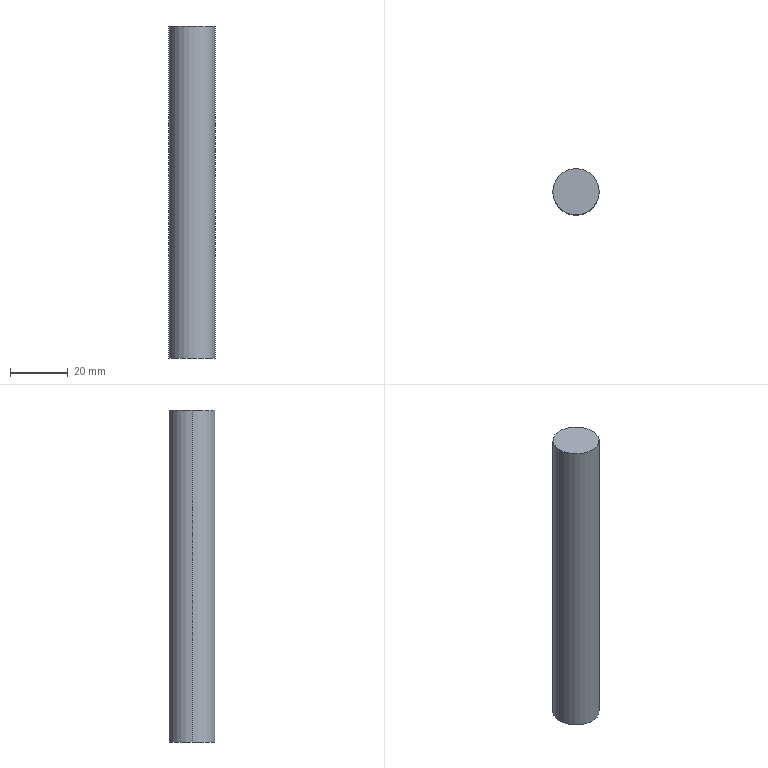Part | STEP file | Support rod | 1 solid | 4 faces | box 16 x 16 x 114.75 mm | volume 23072 mm3 | cylinder 2 | plane 2 | commonest cylinder face diameters 16 x2
STEP:
#1=CARTESIAN_POINT('',(0.,0.,0.));
#2=DIRECTION('',(0.,0.,1.));
#3=DIRECTION('',(1.,0.,0.));
#4=AXIS2_PLACEMENT_3D('',#1,#2,#3);
#5=CARTESIAN_POINT('',(-8.,0.,114.75));
#6=VERTEX_POINT('',#5);
#7=CARTESIAN_POINT('',(8.,0.,114.75));
#8=VERTEX_POINT('',#7);
#9=CARTESIAN_POINT('',(0.,0.,114.75));
#10=DIRECTION('',(0.,0.,-1.));
#11=DIRECTION('',(-1.,0.,0.));
#12=AXIS2_PLACEMENT_3D('',#9,#10,#11);
#13=CIRCLE('',#12,8.);
#14=CARTESIAN_POINT('',(0.,0.,114.75));
#15=DIRECTION('',(0.,0.,-1.));
#16=DIRECTION('',(-1.,0.,0.));
#17=AXIS2_PLACEMENT_3D('',#14,#15,#16);
#18=CYLINDRICAL_SURFACE('',#17,8.);
#19=CARTESIAN_POINT('',(0.,0.));
#20=DIRECTION('',(1.,0.));
#21=VECTOR('',#20,1.);
#22=LINE('',#19,#21);
#23=(GEOMETRIC_REPRESENTATION_CONTEXT(2)PARAMETRIC_REPRESENTATION_CONTEXT()REPRESENTATION_CONTEXT('',''));
#24=DEFINITIONAL_REPRESENTATION('',(#22),#23);
#25=PCURVE('',#18,#24);
#26=CARTESIAN_POINT('',(0.,0.,114.75));
#27=DIRECTION('',(0.,0.,1.));
#28=DIRECTION('',(1.,0.,0.));
#29=AXIS2_PLACEMENT_3D('',#26,#27,#28);
#30=PLANE('',#29);
#31=CARTESIAN_POINT('',(-8.,0.));
#32=CARTESIAN_POINT('',(-8.,13.856));
#33=CARTESIAN_POINT('',(4.,6.928));
#34=CARTESIAN_POINT('',(16.,0.));
#35=CARTESIAN_POINT('',(4.,-6.928));
#36=CARTESIAN_POINT('',(-8.,-13.856));
#37=CARTESIAN_POINT('',(-8.,0.));
#38=(BOUNDED_CURVE()B_SPLINE_CURVE(2,(#31,#32,#33,#34,#35,#36,#37),.UNSPECIFIED.,.T.,.F.)B_SPLINE_CURVE_WITH_KNOTS((1,2,2,2,2,1),(-2.094,0.,2.094,4.189,6.283,8.378),.UNSPECIFIED.)CURVE()GEOMETRIC_REPRESENTATION_ITEM()RATIONAL_B_SPLINE_CURVE((1.,0.5,1.,0.5,1.,0.5,1.))REPRESENTATION_ITEM(''));
#39=(GEOMETRIC_REPRESENTATION_CONTEXT(2)PARAMETRIC_REPRESENTATION_CONTEXT()REPRESENTATION_CONTEXT('',''));
#40=DEFINITIONAL_REPRESENTATION('',(#38),#39);
#41=PCURVE('',#30,#40);
#42=SURFACE_CURVE('',#13,(#25,#41),.PCURVE_S1.);
#43=EDGE_CURVE('',#6,#8,#42,.T.);
#44=ORIENTED_EDGE('',*,*,#43,.T.);
#45=CARTESIAN_POINT('',(8.,0.,0.));
#46=VERTEX_POINT('',#45);
#47=CARTESIAN_POINT('',(8.,0.,114.75));
#48=DIRECTION('',(0.,0.,-1.));
#49=VECTOR('',#48,1.);
#50=LINE('',#47,#49);
#51=CARTESIAN_POINT('',(3.142,0.));
#52=DIRECTION('',(0.,1.));
#53=VECTOR('',#52,1.);
#54=LINE('',#51,#53);
#55=(GEOMETRIC_REPRESENTATION_CONTEXT(2)PARAMETRIC_REPRESENTATION_CONTEXT()REPRESENTATION_CONTEXT('',''));
#56=DEFINITIONAL_REPRESENTATION('',(#54),#55);
#57=PCURVE('',#18,#56);
#58=CARTESIAN_POINT('',(0.,0.,114.75));
#59=DIRECTION('',(0.,0.,-1.));
#60=DIRECTION('',(-1.,0.,0.));
#61=AXIS2_PLACEMENT_3D('',#58,#59,#60);
#62=CYLINDRICAL_SURFACE('',#61,8.);
#63=CARTESIAN_POINT('',(3.142,0.));
#64=DIRECTION('',(0.,1.));
#65=VECTOR('',#64,1.);
#66=LINE('',#63,#65);
#67=(GEOMETRIC_REPRESENTATION_CONTEXT(2)PARAMETRIC_REPRESENTATION_CONTEXT()REPRESENTATION_CONTEXT('',''));
#68=DEFINITIONAL_REPRESENTATION('',(#66),#67);
#69=PCURVE('',#62,#68);
#70=SURFACE_CURVE('',#50,(#57,#69),.PCURVE_S1.);
#71=EDGE_CURVE('',#8,#46,#70,.T.);
#72=ORIENTED_EDGE('',*,*,#71,.T.);
#73=CARTESIAN_POINT('',(-8.,0.,0.));
#74=VERTEX_POINT('',#73);
#75=CARTESIAN_POINT('',(0.,0.,0.));
#76=DIRECTION('',(0.,0.,1.));
#77=DIRECTION('',(-1.,0.,0.));
#78=AXIS2_PLACEMENT_3D('',#75,#76,#77);
#79=CIRCLE('',#78,8.);
#80=CARTESIAN_POINT('',(6.283,114.75));
#81=DIRECTION('',(-1.,0.));
#82=VECTOR('',#81,1.);
#83=LINE('',#80,#82);
#84=(GEOMETRIC_REPRESENTATION_CONTEXT(2)PARAMETRIC_REPRESENTATION_CONTEXT()REPRESENTATION_CONTEXT('',''));
#85=DEFINITIONAL_REPRESENTATION('',(#83),#84);
#86=PCURVE('',#18,#85);
#87=CARTESIAN_POINT('',(0.,0.,0.));
#88=DIRECTION('',(0.,0.,1.));
#89=DIRECTION('',(1.,0.,0.));
#90=AXIS2_PLACEMENT_3D('',#87,#88,#89);
#91=PLANE('',#90);
#92=CARTESIAN_POINT('',(0.,0.));
#93=DIRECTION('',(-1.,0.));
#94=AXIS2_PLACEMENT_2D('',#92,#93);
#95=CIRCLE('',#94,8.);
#96=(GEOMETRIC_REPRESENTATION_CONTEXT(2)PARAMETRIC_REPRESENTATION_CONTEXT()REPRESENTATION_CONTEXT('',''));
#97=DEFINITIONAL_REPRESENTATION('',(#95),#96);
#98=PCURVE('',#91,#97);
#99=SURFACE_CURVE('',#79,(#86,#98),.PCURVE_S1.);
#100=EDGE_CURVE('',#46,#74,#99,.T.);
#101=ORIENTED_EDGE('',*,*,#100,.T.);
#102=CARTESIAN_POINT('',(-8.,0.,114.75));
#103=DIRECTION('',(0.,0.,-1.));
#104=VECTOR('',#103,1.);
#105=LINE('',#102,#104);
#106=CARTESIAN_POINT('',(0.,0.));
#107=DIRECTION('',(0.,1.));
#108=VECTOR('',#107,1.);
#109=LINE('',#106,#108);
#110=(GEOMETRIC_REPRESENTATION_CONTEXT(2)PARAMETRIC_REPRESENTATION_CONTEXT()REPRESENTATION_CONTEXT('',''));
#111=DEFINITIONAL_REPRESENTATION('',(#109),#110);
#112=PCURVE('',#18,#111);
#113=CARTESIAN_POINT('',(6.283,0.));
#114=DIRECTION('',(0.,1.));
#115=VECTOR('',#114,1.);
#116=LINE('',#113,#115);
#117=(GEOMETRIC_REPRESENTATION_CONTEXT(2)PARAMETRIC_REPRESENTATION_CONTEXT()REPRESENTATION_CONTEXT('',''));
#118=DEFINITIONAL_REPRESENTATION('',(#116),#117);
#119=PCURVE('',#62,#118);
#120=SURFACE_CURVE('',#105,(#112,#119),.PCURVE_S1.);
#121=EDGE_CURVE('',#6,#74,#120,.T.);
#122=ORIENTED_EDGE('',*,*,#121,.F.);
#123=EDGE_LOOP('',(#44,#72,#101,#122));
#124=FACE_BOUND('',#123,.T.);
#125=ADVANCED_FACE('',(#124),#18,.T.);
#126=ORIENTED_EDGE('',*,*,#71,.F.);
#127=CARTESIAN_POINT('',(0.,0.,114.75));
#128=DIRECTION('',(0.,0.,-1.));
#129=DIRECTION('',(-1.,0.,0.));
#130=AXIS2_PLACEMENT_3D('',#127,#128,#129);
#131=CIRCLE('',#130,8.);
#132=CARTESIAN_POINT('',(0.,0.));
#133=DIRECTION('',(1.,0.));
#134=VECTOR('',#133,1.);
#135=LINE('',#132,#134);
#136=(GEOMETRIC_REPRESENTATION_CONTEXT(2)PARAMETRIC_REPRESENTATION_CONTEXT()REPRESENTATION_CONTEXT('',''));
#137=DEFINITIONAL_REPRESENTATION('',(#135),#136);
#138=PCURVE('',#62,#137);
#139=CARTESIAN_POINT('',(-8.,0.));
#140=CARTESIAN_POINT('',(-8.,13.856));
#141=CARTESIAN_POINT('',(4.,6.928));
#142=CARTESIAN_POINT('',(16.,0.));
#143=CARTESIAN_POINT('',(4.,-6.928));
#144=CARTESIAN_POINT('',(-8.,-13.856));
#145=CARTESIAN_POINT('',(-8.,0.));
#146=(BOUNDED_CURVE()B_SPLINE_CURVE(2,(#139,#140,#141,#142,#143,#144,#145),.UNSPECIFIED.,.T.,.F.)B_SPLINE_CURVE_WITH_KNOTS((1,2,2,2,2,1),(-2.094,0.,2.094,4.189,6.283,8.378),.UNSPECIFIED.)CURVE()GEOMETRIC_REPRESENTATION_ITEM()RATIONAL_B_SPLINE_CURVE((1.,0.5,1.,0.5,1.,0.5,1.))REPRESENTATION_ITEM(''));
#147=(GEOMETRIC_REPRESENTATION_CONTEXT(2)PARAMETRIC_REPRESENTATION_CONTEXT()REPRESENTATION_CONTEXT('',''));
#148=DEFINITIONAL_REPRESENTATION('',(#146),#147);
#149=PCURVE('',#30,#148);
#150=SURFACE_CURVE('',#131,(#138,#149),.PCURVE_S1.);
#151=EDGE_CURVE('',#8,#6,#150,.T.);
#152=ORIENTED_EDGE('',*,*,#151,.T.);
#153=ORIENTED_EDGE('',*,*,#121,.T.);
#154=CARTESIAN_POINT('',(0.,0.,0.));
#155=DIRECTION('',(0.,0.,1.));
#156=DIRECTION('',(-1.,0.,0.));
#157=AXIS2_PLACEMENT_3D('',#154,#155,#156);
#158=CIRCLE('',#157,8.);
#159=CARTESIAN_POINT('',(6.283,114.75));
#160=DIRECTION('',(-1.,0.));
#161=VECTOR('',#160,1.);
#162=LINE('',#159,#161);
#163=(GEOMETRIC_REPRESENTATION_CONTEXT(2)PARAMETRIC_REPRESENTATION_CONTEXT()REPRESENTATION_CONTEXT('',''));
#164=DEFINITIONAL_REPRESENTATION('',(#162),#163);
#165=PCURVE('',#62,#164);
#166=CARTESIAN_POINT('',(0.,0.));
#167=DIRECTION('',(-1.,0.));
#168=AXIS2_PLACEMENT_2D('',#166,#167);
#169=CIRCLE('',#168,8.);
#170=(GEOMETRIC_REPRESENTATION_CONTEXT(2)PARAMETRIC_REPRESENTATION_CONTEXT()REPRESENTATION_CONTEXT('',''));
#171=DEFINITIONAL_REPRESENTATION('',(#169),#170);
#172=PCURVE('',#91,#171);
#173=SURFACE_CURVE('',#158,(#165,#172),.PCURVE_S1.);
#174=EDGE_CURVE('',#74,#46,#173,.T.);
#175=ORIENTED_EDGE('',*,*,#174,.T.);
#176=EDGE_LOOP('',(#126,#152,#153,#175));
#177=FACE_BOUND('',#176,.T.);
#178=ADVANCED_FACE('',(#177),#62,.T.);
#179=ORIENTED_EDGE('',*,*,#174,.F.);
#180=ORIENTED_EDGE('',*,*,#100,.F.);
#181=EDGE_LOOP('',(#179,#180));
#182=FACE_BOUND('',#181,.T.);
#183=ADVANCED_FACE('',(#182),#91,.F.);
#184=ORIENTED_EDGE('',*,*,#43,.F.);
#185=ORIENTED_EDGE('',*,*,#151,.F.);
#186=EDGE_LOOP('',(#184,#185));
#187=FACE_BOUND('',#186,.T.);
#188=ADVANCED_FACE('',(#187),#30,.T.);
#189=CLOSED_SHELL('',(#125,#178,#183,#188));
#190=MANIFOLD_SOLID_BREP('',#189);
#191=(LENGTH_UNIT()NAMED_UNIT(*)SI_UNIT(.MILLI.,.METRE.));
#192=UNCERTAINTY_MEASURE_WITH_UNIT(LENGTH_MEASURE(0.0000001),#191,'','');
#193=(NAMED_UNIT(*)PLANE_ANGLE_UNIT()SI_UNIT($,.RADIAN.));
#194=(NAMED_UNIT(*)SI_UNIT($,.STERADIAN.)SOLID_ANGLE_UNIT());
#195=(GEOMETRIC_REPRESENTATION_CONTEXT(3)GLOBAL_UNCERTAINTY_ASSIGNED_CONTEXT((#192))GLOBAL_UNIT_ASSIGNED_CONTEXT((#191,#193,#194))REPRESENTATION_CONTEXT('',''));
#196=ADVANCED_BREP_SHAPE_REPRESENTATION('',(#4,#190),#195);